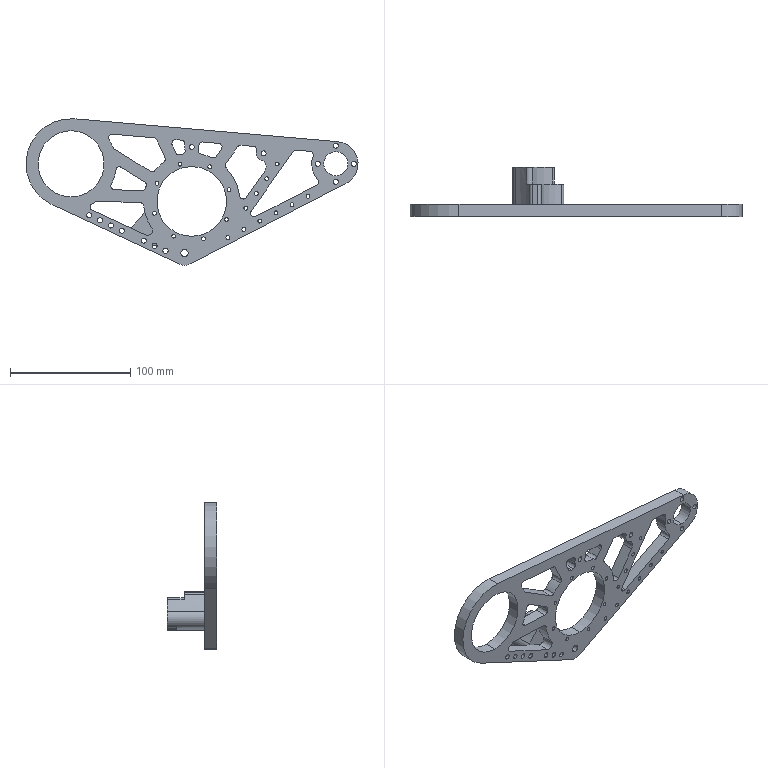Part | SolidWorks | features ICE 8, Fillet 5, Extrusion 1, MirrorSolid 1 | 2 solids | 174 faces | box 276 x 41 x 121.736 mm | volume 133233 mm3 | cylinder 145 | plane 29 | commonest cylinder face diameters 6 x46 3.2 x40 4.2 x28 80 x6 12 x4 20 x4